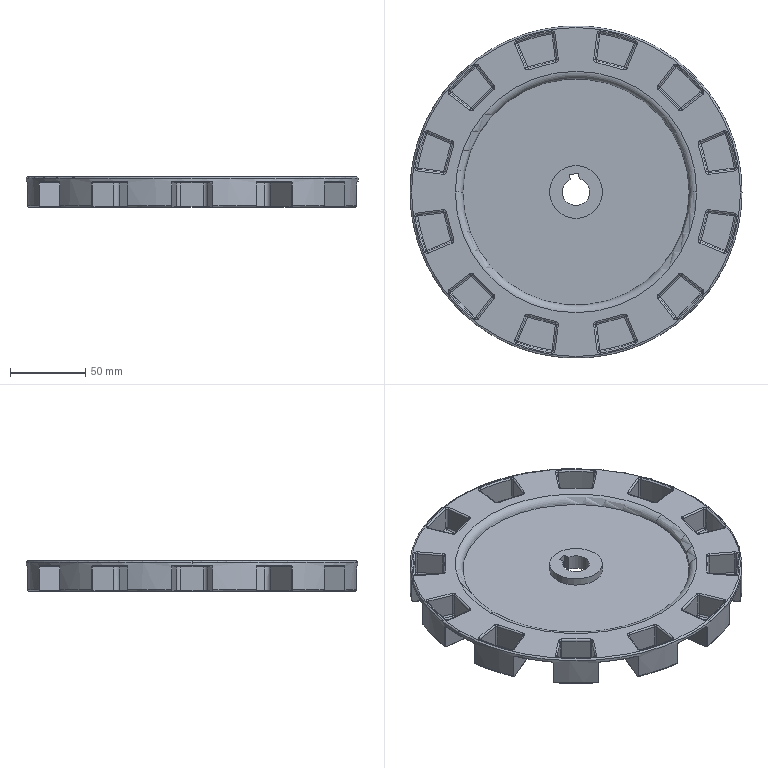Part | SolidWorks | features Fillet 5, ICE 5, CirPattern 2, Revolution 1 | 1 solid | 666 faces | box 220 x 220 x 20 mm | volume 250365 mm3 | cylinder 281 | torus 173 | plane 104 | sphere 60 | spline 48 | commonest cylinder face diameters 2 x166 0.4 x66 6 x28 214 x12 18 x3 35 x2